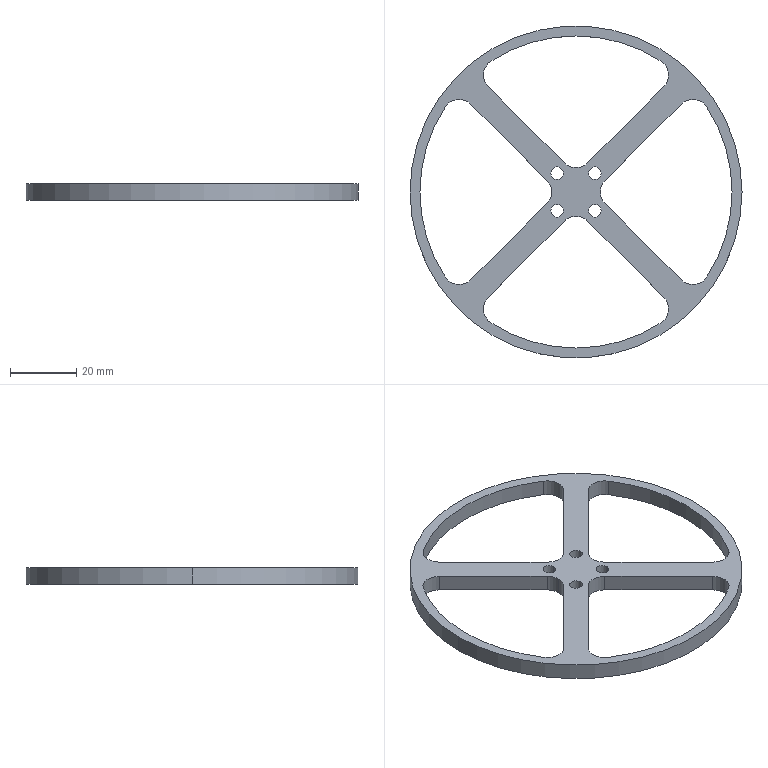Part | SolidWorks | features Cut 1, Extrusion 1, Fillet 1 | 1 solid | 40 faces | box 100 x 100 x 5 mm | volume 11461 mm3 | cylinder 30 | plane 10 | commonest cylinder face diameters 10 x15 3.8 x8 94 x5 100 x2
STEP:
#1=CARTESIAN_POINT('',(-7.557,-5.657,0.));
#2=VERTEX_POINT('',#1);
#3=CARTESIAN_POINT('',(-3.757,-5.657,0.));
#4=VERTEX_POINT('',#3);
#5=CARTESIAN_POINT('',(-5.657,-5.657,0.));
#6=DIRECTION('',(0.,0.,1.));
#7=DIRECTION('',(1.,0.,0.));
#8=AXIS2_PLACEMENT_3D('',#5,#6,#7);
#9=CIRCLE('',#8,1.9);
#10=EDGE_CURVE('',#2,#4,#9,.T.);
#11=ORIENTED_EDGE('',*,*,#10,.F.);
#12=CARTESIAN_POINT('',(-7.557,-5.657,5.));
#13=VERTEX_POINT('',#12);
#14=CARTESIAN_POINT('',(-7.557,-5.657,0.));
#15=DIRECTION('',(0.,0.,1.));
#16=VECTOR('',#15,1000.);
#17=LINE('',#14,#16);
#18=EDGE_CURVE('',#2,#13,#17,.T.);
#19=ORIENTED_EDGE('',*,*,#18,.T.);
#20=CARTESIAN_POINT('',(-3.757,-5.657,5.));
#21=VERTEX_POINT('',#20);
#22=CARTESIAN_POINT('',(-5.657,-5.657,5.));
#23=DIRECTION('',(0.,0.,1.));
#24=DIRECTION('',(1.,0.,0.));
#25=AXIS2_PLACEMENT_3D('',#22,#23,#24);
#26=CIRCLE('',#25,1.9);
#27=EDGE_CURVE('',#13,#21,#26,.T.);
#28=ORIENTED_EDGE('',*,*,#27,.T.);
#29=CARTESIAN_POINT('',(-3.757,-5.657,0.));
#30=DIRECTION('',(0.,0.,1.));
#31=VECTOR('',#30,1000.);
#32=LINE('',#29,#31);
#33=EDGE_CURVE('',#4,#21,#32,.T.);
#34=ORIENTED_EDGE('',*,*,#33,.F.);
#35=EDGE_LOOP('',(#11,#19,#28,#34));
#36=FACE_OUTER_BOUND('',#35,.T.);
#37=CARTESIAN_POINT('',(-5.657,-5.657,0.));
#38=DIRECTION('',(0.,0.,1.));
#39=DIRECTION('',(1.,0.,0.));
#40=AXIS2_PLACEMENT_3D('',#37,#38,#39);
#41=CYLINDRICAL_SURFACE('',#40,1.9);
#42=ADVANCED_FACE('',(#36),#41,.F.);
#43=CARTESIAN_POINT('',(-7.557,5.657,0.));
#44=VERTEX_POINT('',#43);
#45=CARTESIAN_POINT('',(-3.757,5.657,0.));
#46=VERTEX_POINT('',#45);
#47=CARTESIAN_POINT('',(-5.657,5.657,0.));
#48=DIRECTION('',(0.,0.,1.));
#49=DIRECTION('',(1.,0.,0.));
#50=AXIS2_PLACEMENT_3D('',#47,#48,#49);
#51=CIRCLE('',#50,1.9);
#52=EDGE_CURVE('',#44,#46,#51,.T.);
#53=ORIENTED_EDGE('',*,*,#52,.F.);
#54=CARTESIAN_POINT('',(-7.557,5.657,5.));
#55=VERTEX_POINT('',#54);
#56=CARTESIAN_POINT('',(-7.557,5.657,0.));
#57=DIRECTION('',(0.,0.,1.));
#58=VECTOR('',#57,1000.);
#59=LINE('',#56,#58);
#60=EDGE_CURVE('',#44,#55,#59,.T.);
#61=ORIENTED_EDGE('',*,*,#60,.T.);
#62=CARTESIAN_POINT('',(-3.757,5.657,5.));
#63=VERTEX_POINT('',#62);
#64=CARTESIAN_POINT('',(-5.657,5.657,5.));
#65=DIRECTION('',(0.,0.,1.));
#66=DIRECTION('',(1.,0.,0.));
#67=AXIS2_PLACEMENT_3D('',#64,#65,#66);
#68=CIRCLE('',#67,1.9);
#69=EDGE_CURVE('',#55,#63,#68,.T.);
#70=ORIENTED_EDGE('',*,*,#69,.T.);
#71=CARTESIAN_POINT('',(-3.757,5.657,0.));
#72=DIRECTION('',(0.,0.,1.));
#73=VECTOR('',#72,1000.);
#74=LINE('',#71,#73);
#75=EDGE_CURVE('',#46,#63,#74,.T.);
#76=ORIENTED_EDGE('',*,*,#75,.F.);
#77=EDGE_LOOP('',(#53,#61,#70,#76));
#78=FACE_OUTER_BOUND('',#77,.T.);
#79=CARTESIAN_POINT('',(-5.657,5.657,0.));
#80=DIRECTION('',(0.,0.,1.));
#81=DIRECTION('',(1.,0.,0.));
#82=AXIS2_PLACEMENT_3D('',#79,#80,#81);
#83=CYLINDRICAL_SURFACE('',#82,1.9);
#84=ADVANCED_FACE('',(#78),#83,.F.);
#85=CARTESIAN_POINT('',(3.757,5.657,0.));
#86=VERTEX_POINT('',#85);
#87=CARTESIAN_POINT('',(7.557,5.657,0.));
#88=VERTEX_POINT('',#87);
#89=CARTESIAN_POINT('',(5.657,5.657,0.));
#90=DIRECTION('',(0.,0.,1.));
#91=DIRECTION('',(1.,0.,0.));
#92=AXIS2_PLACEMENT_3D('',#89,#90,#91);
#93=CIRCLE('',#92,1.9);
#94=EDGE_CURVE('',#86,#88,#93,.T.);
#95=ORIENTED_EDGE('',*,*,#94,.F.);
#96=CARTESIAN_POINT('',(3.757,5.657,5.));
#97=VERTEX_POINT('',#96);
#98=CARTESIAN_POINT('',(3.757,5.657,0.));
#99=DIRECTION('',(0.,0.,1.));
#100=VECTOR('',#99,1000.);
#101=LINE('',#98,#100);
#102=EDGE_CURVE('',#86,#97,#101,.T.);
#103=ORIENTED_EDGE('',*,*,#102,.T.);
#104=CARTESIAN_POINT('',(7.557,5.657,5.));
#105=VERTEX_POINT('',#104);
#106=CARTESIAN_POINT('',(5.657,5.657,5.));
#107=DIRECTION('',(0.,0.,1.));
#108=DIRECTION('',(1.,0.,0.));
#109=AXIS2_PLACEMENT_3D('',#106,#107,#108);
#110=CIRCLE('',#109,1.9);
#111=EDGE_CURVE('',#97,#105,#110,.T.);
#112=ORIENTED_EDGE('',*,*,#111,.T.);
#113=CARTESIAN_POINT('',(7.557,5.657,0.));
#114=DIRECTION('',(0.,0.,1.));
#115=VECTOR('',#114,1000.);
#116=LINE('',#113,#115);
#117=EDGE_CURVE('',#88,#105,#116,.T.);
#118=ORIENTED_EDGE('',*,*,#117,.F.);
#119=EDGE_LOOP('',(#95,#103,#112,#118));
#120=FACE_OUTER_BOUND('',#119,.T.);
#121=CARTESIAN_POINT('',(5.657,5.657,0.));
#122=DIRECTION('',(0.,0.,1.));
#123=DIRECTION('',(1.,0.,0.));
#124=AXIS2_PLACEMENT_3D('',#121,#122,#123);
#125=CYLINDRICAL_SURFACE('',#124,1.9);
#126=ADVANCED_FACE('',(#120),#125,.F.);
#127=CARTESIAN_POINT('',(3.757,-5.657,0.));
#128=VERTEX_POINT('',#127);
#129=CARTESIAN_POINT('',(7.557,-5.657,0.));
#130=VERTEX_POINT('',#129);
#131=CARTESIAN_POINT('',(5.657,-5.657,0.));
#132=DIRECTION('',(0.,0.,1.));
#133=DIRECTION('',(1.,0.,0.));
#134=AXIS2_PLACEMENT_3D('',#131,#132,#133);
#135=CIRCLE('',#134,1.9);
#136=EDGE_CURVE('',#128,#130,#135,.T.);
#137=ORIENTED_EDGE('',*,*,#136,.F.);
#138=CARTESIAN_POINT('',(3.757,-5.657,5.));
#139=VERTEX_POINT('',#138);
#140=CARTESIAN_POINT('',(3.757,-5.657,0.));
#141=DIRECTION('',(0.,0.,1.));
#142=VECTOR('',#141,1000.);
#143=LINE('',#140,#142);
#144=EDGE_CURVE('',#128,#139,#143,.T.);
#145=ORIENTED_EDGE('',*,*,#144,.T.);
#146=CARTESIAN_POINT('',(7.557,-5.657,5.));
#147=VERTEX_POINT('',#146);
#148=CARTESIAN_POINT('',(5.657,-5.657,5.));
#149=DIRECTION('',(0.,0.,1.));
#150=DIRECTION('',(1.,0.,0.));
#151=AXIS2_PLACEMENT_3D('',#148,#149,#150);
#152=CIRCLE('',#151,1.9);
#153=EDGE_CURVE('',#139,#147,#152,.T.);
#154=ORIENTED_EDGE('',*,*,#153,.T.);
#155=CARTESIAN_POINT('',(7.557,-5.657,0.));
#156=DIRECTION('',(0.,0.,1.));
#157=VECTOR('',#156,1000.);
#158=LINE('',#155,#157);
#159=EDGE_CURVE('',#130,#147,#158,.T.);
#160=ORIENTED_EDGE('',*,*,#159,.F.);
#161=EDGE_LOOP('',(#137,#145,#154,#160));
#162=FACE_OUTER_BOUND('',#161,.T.);
#163=CARTESIAN_POINT('',(5.657,-5.657,0.));
#164=DIRECTION('',(0.,0.,1.));
#165=DIRECTION('',(1.,0.,0.));
#166=AXIS2_PLACEMENT_3D('',#163,#164,#165);
#167=CYLINDRICAL_SURFACE('',#166,1.9);
#168=ADVANCED_FACE('',(#162),#167,.F.);
#169=CARTESIAN_POINT('',(-27.891,35.214,5.));
#170=VERTEX_POINT('',#169);
#171=CARTESIAN_POINT('',(-25.616,39.406,5.));
#172=VERTEX_POINT('',#171);
#173=CARTESIAN_POINT('',(-22.891,35.214,5.));
#174=DIRECTION('',(0.,0.,-1.));
#175=DIRECTION('',(1.,0.,0.));
#176=AXIS2_PLACEMENT_3D('',#173,#174,#175);
#177=CIRCLE('',#176,5.);
#178=EDGE_CURVE('',#170,#172,#177,.T.);
#179=ORIENTED_EDGE('',*,*,#178,.F.);
#180=CARTESIAN_POINT('',(-27.891,35.214,0.));
#181=VERTEX_POINT('',#180);
#182=CARTESIAN_POINT('',(-27.891,35.214,5.));
#183=DIRECTION('',(0.,0.,-1.));
#184=VECTOR('',#183,1000.);
#185=LINE('',#182,#184);
#186=EDGE_CURVE('',#170,#181,#185,.T.);
#187=ORIENTED_EDGE('',*,*,#186,.T.);
#188=CARTESIAN_POINT('',(-25.616,39.406,0.));
#189=VERTEX_POINT('',#188);
#190=CARTESIAN_POINT('',(-22.891,35.214,0.));
#191=DIRECTION('',(0.,0.,1.));
#192=DIRECTION('',(1.,0.,0.));
#193=AXIS2_PLACEMENT_3D('',#190,#191,#192);
#194=CIRCLE('',#193,5.);
#195=EDGE_CURVE('',#189,#181,#194,.T.);
#196=ORIENTED_EDGE('',*,*,#195,.F.);
#197=CARTESIAN_POINT('',(-25.616,39.406,5.));
#198=DIRECTION('',(0.,0.,-1.));
#199=VECTOR('',#198,1000.);
#200=LINE('',#197,#199);
#201=EDGE_CURVE('',#172,#189,#200,.T.);
#202=ORIENTED_EDGE('',*,*,#201,.F.);
#203=EDGE_LOOP('',(#179,#187,#196,#202));
#204=FACE_OUTER_BOUND('',#203,.T.);
#205=CARTESIAN_POINT('',(-22.891,35.214,5.));
#206=DIRECTION('',(0.,0.,-1.));
#207=DIRECTION('',(-1.,0.,0.));
#208=AXIS2_PLACEMENT_3D('',#205,#206,#207);
#209=CYLINDRICAL_SURFACE('',#208,5.);
#210=ADVANCED_FACE('',(#204),#209,.F.);
#211=CARTESIAN_POINT('',(-27.891,-35.214,5.));
#212=VERTEX_POINT('',#211);
#213=CARTESIAN_POINT('',(-26.427,-31.678,5.));
#214=VERTEX_POINT('',#213);
#215=CARTESIAN_POINT('',(-22.891,-35.214,5.));
#216=DIRECTION('',(0.,0.,-1.));
#217=DIRECTION('',(1.,0.,0.));
#218=AXIS2_PLACEMENT_3D('',#215,#216,#217);
#219=CIRCLE('',#218,5.);
#220=EDGE_CURVE('',#212,#214,#219,.T.);
#221=ORIENTED_EDGE('',*,*,#220,.F.);
#222=CARTESIAN_POINT('',(-27.891,-35.214,0.));
#223=VERTEX_POINT('',#222);
#224=CARTESIAN_POINT('',(-27.891,-35.214,5.));
#225=DIRECTION('',(0.,0.,-1.));
#226=VECTOR('',#225,1000.);
#227=LINE('',#224,#226);
#228=EDGE_CURVE('',#212,#223,#227,.T.);
#229=ORIENTED_EDGE('',*,*,#228,.T.);
#230=CARTESIAN_POINT('',(-26.427,-31.678,0.));
#231=VERTEX_POINT('',#230);
#232=CARTESIAN_POINT('',(-22.891,-35.214,0.));
#233=DIRECTION('',(0.,0.,1.));
#234=DIRECTION('',(1.,0.,0.));
#235=AXIS2_PLACEMENT_3D('',#232,#233,#234);
#236=CIRCLE('',#235,5.);
#237=EDGE_CURVE('',#231,#223,#236,.T.);
#238=ORIENTED_EDGE('',*,*,#237,.F.);
#239=CARTESIAN_POINT('',(-26.427,-31.678,0.));
#240=DIRECTION('',(0.,0.,-1.));
#241=VECTOR('',#240,1000.);
#242=LINE('',#239,#241);
#243=EDGE_CURVE('',#214,#231,#242,.T.);
#244=ORIENTED_EDGE('',*,*,#243,.F.);
#245=EDGE_LOOP('',(#221,#229,#238,#244));
#246=FACE_OUTER_BOUND('',#245,.T.);
#247=CARTESIAN_POINT('',(-22.891,-35.214,5.));
#248=DIRECTION('',(0.,0.,-1.));
#249=DIRECTION('',(-1.,0.,0.));
#250=AXIS2_PLACEMENT_3D('',#247,#248,#249);
#251=CYLINDRICAL_SURFACE('',#250,5.);
#252=ADVANCED_FACE('',(#246),#251,.F.);
#253=CARTESIAN_POINT('',(-7.322,0.,0.));
#254=VERTEX_POINT('',#253);
#255=CARTESIAN_POINT('',(-8.787,3.536,0.));
#256=VERTEX_POINT('',#255);
#257=CARTESIAN_POINT('',(-12.322,0.,0.));
#258=DIRECTION('',(0.,0.,1.));
#259=DIRECTION('',(1.,0.,0.));
#260=AXIS2_PLACEMENT_3D('',#257,#258,#259);
#261=CIRCLE('',#260,5.);
#262=EDGE_CURVE('',#254,#256,#261,.T.);
#263=ORIENTED_EDGE('',*,*,#262,.F.);
#264=CARTESIAN_POINT('',(-7.322,0.,5.));
#265=VERTEX_POINT('',#264);
#266=CARTESIAN_POINT('',(-7.322,0.,5.));
#267=DIRECTION('',(0.,0.,1.));
#268=VECTOR('',#267,1000.);
#269=LINE('',#266,#268);
#270=EDGE_CURVE('',#254,#265,#269,.T.);
#271=ORIENTED_EDGE('',*,*,#270,.T.);
#272=CARTESIAN_POINT('',(-8.787,3.536,5.));
#273=VERTEX_POINT('',#272);
#274=CARTESIAN_POINT('',(-12.322,0.,5.));
#275=DIRECTION('',(0.,0.,-1.));
#276=DIRECTION('',(1.,0.,0.));
#277=AXIS2_PLACEMENT_3D('',#274,#275,#276);
#278=CIRCLE('',#277,5.);
#279=EDGE_CURVE('',#273,#265,#278,.T.);
#280=ORIENTED_EDGE('',*,*,#279,.F.);
#281=CARTESIAN_POINT('',(-8.787,3.536,5.));
#282=DIRECTION('',(0.,0.,1.));
#283=VECTOR('',#282,1000.);
#284=LINE('',#281,#283);
#285=EDGE_CURVE('',#256,#273,#284,.T.);
#286=ORIENTED_EDGE('',*,*,#285,.F.);
#287=EDGE_LOOP('',(#263,#271,#280,#286));
#288=FACE_OUTER_BOUND('',#287,.T.);
#289=CARTESIAN_POINT('',(-12.322,0.,5.));
#290=DIRECTION('',(0.,0.,1.));
#291=DIRECTION('',(1.,0.,0.));
#292=AXIS2_PLACEMENT_3D('',#289,#290,#291);
#293=CYLINDRICAL_SURFACE('',#292,5.);
#294=ADVANCED_FACE('',(#288),#293,.F.);
#295=CARTESIAN_POINT('',(-39.406,25.616,5.));
#296=VERTEX_POINT('',#295);
#297=CARTESIAN_POINT('',(-47.,0.,5.));
#298=VERTEX_POINT('',#297);
#299=CARTESIAN_POINT('',(0.,0.,5.));
#300=DIRECTION('',(0.,0.,1.));
#301=DIRECTION('',(1.,0.,0.));
#302=AXIS2_PLACEMENT_3D('',#299,#300,#301);
#303=CIRCLE('',#302,47.);
#304=EDGE_CURVE('',#296,#298,#303,.T.);
#305=ORIENTED_EDGE('',*,*,#304,.T.);
#306=CARTESIAN_POINT('',(-47.,0.,0.));
#307=VERTEX_POINT('',#306);
#308=CARTESIAN_POINT('',(-47.,0.,5.));
#309=DIRECTION('',(0.,0.,-1.));
#310=VECTOR('',#309,1000.);
#311=LINE('',#308,#310);
#312=EDGE_CURVE('',#298,#307,#311,.T.);
#313=ORIENTED_EDGE('',*,*,#312,.T.);
#314=CARTESIAN_POINT('',(-39.406,25.616,0.));
#315=VERTEX_POINT('',#314);
#316=CARTESIAN_POINT('',(0.,0.,0.));
#317=DIRECTION('',(0.,0.,1.));
#318=DIRECTION('',(1.,0.,0.));
#319=AXIS2_PLACEMENT_3D('',#316,#317,#318);
#320=CIRCLE('',#319,47.);
#321=EDGE_CURVE('',#315,#307,#320,.T.);
#322=ORIENTED_EDGE('',*,*,#321,.F.);
#323=CARTESIAN_POINT('',(-39.406,25.616,5.));
#324=DIRECTION('',(0.,0.,1.));
#325=VECTOR('',#324,1000.);
#326=LINE('',#323,#325);
#327=EDGE_CURVE('',#315,#296,#326,.T.);
#328=ORIENTED_EDGE('',*,*,#327,.T.);
#329=EDGE_LOOP('',(#305,#313,#322,#328));
#330=FACE_OUTER_BOUND('',#329,.T.);
#331=CARTESIAN_POINT('',(0.,0.,5.));
#332=DIRECTION('',(0.,0.,-1.));
#333=DIRECTION('',(-1.,0.,0.));
#334=AXIS2_PLACEMENT_3D('',#331,#332,#333);
#335=CYLINDRICAL_SURFACE('',#334,47.);
#336=ADVANCED_FACE('',(#330),#335,.F.);
#337=CARTESIAN_POINT('',(50.,0.,5.));
#338=VERTEX_POINT('',#337);
#339=CARTESIAN_POINT('',(-50.,0.,5.));
#340=VERTEX_POINT('',#339);
#341=CARTESIAN_POINT('',(0.,0.,5.));
#342=DIRECTION('',(0.,0.,1.));
#343=DIRECTION('',(1.,0.,0.));
#344=AXIS2_PLACEMENT_3D('',#341,#342,#343);
#345=CIRCLE('',#344,50.);
#346=EDGE_CURVE('',#338,#340,#345,.T.);
#347=ORIENTED_EDGE('',*,*,#346,.F.);
#348=CARTESIAN_POINT('',(50.,0.,0.));
#349=VERTEX_POINT('',#348);
#350=CARTESIAN_POINT('',(50.,0.,5.));
#351=DIRECTION('',(0.,0.,-1.));
#352=VECTOR('',#351,1000.);
#353=LINE('',#350,#352);
#354=EDGE_CURVE('',#338,#349,#353,.T.);
#355=ORIENTED_EDGE('',*,*,#354,.T.);
#356=CARTESIAN_POINT('',(-50.,0.,0.));
#357=VERTEX_POINT('',#356);
#358=CARTESIAN_POINT('',(0.,0.,0.));
#359=DIRECTION('',(0.,0.,1.));
#360=DIRECTION('',(1.,0.,0.));
#361=AXIS2_PLACEMENT_3D('',#358,#359,#360);
#362=CIRCLE('',#361,50.);
#363=EDGE_CURVE('',#349,#357,#362,.T.);
#364=ORIENTED_EDGE('',*,*,#363,.T.);
#365=CARTESIAN_POINT('',(-50.,0.,5.));
#366=DIRECTION('',(0.,0.,-1.));
#367=VECTOR('',#366,1000.);
#368=LINE('',#365,#367);
#369=EDGE_CURVE('',#340,#357,#368,.T.);
#370=ORIENTED_EDGE('',*,*,#369,.F.);
#371=EDGE_LOOP('',(#347,#355,#364,#370));
#372=FACE_OUTER_BOUND('',#371,.T.);
#373=CARTESIAN_POINT('',(0.,0.,5.));
#374=DIRECTION('',(0.,0.,-1.));
#375=DIRECTION('',(-1.,0.,0.));
#376=AXIS2_PLACEMENT_3D('',#373,#374,#375);
#377=CYLINDRICAL_SURFACE('',#376,50.);
#378=ADVANCED_FACE('',(#372),#377,.T.);
#379=CARTESIAN_POINT('',(-5.657,-5.657,5.));
#380=DIRECTION('',(0.,0.,1.));
#381=DIRECTION('',(1.,0.,0.));
#382=AXIS2_PLACEMENT_3D('',#379,#380,#381);
#383=CIRCLE('',#382,1.9);
#384=EDGE_CURVE('',#21,#13,#383,.T.);
#385=ORIENTED_EDGE('',*,*,#384,.F.);
#386=ORIENTED_EDGE('',*,*,#27,.F.);
#387=EDGE_LOOP('',(#385,#386));
#388=FACE_BOUND('',#387,.T.);
#389=CARTESIAN_POINT('',(-5.657,5.657,5.));
#390=DIRECTION('',(0.,0.,1.));
#391=DIRECTION('',(1.,0.,0.));
#392=AXIS2_PLACEMENT_3D('',#389,#390,#391);
#393=CIRCLE('',#392,1.9);
#394=EDGE_CURVE('',#63,#55,#393,.T.);
#395=ORIENTED_EDGE('',*,*,#394,.F.);
#396=ORIENTED_EDGE('',*,*,#69,.F.);
#397=EDGE_LOOP('',(#395,#396));
#398=FACE_BOUND('',#397,.T.);
#399=CARTESIAN_POINT('',(5.657,5.657,5.));
#400=DIRECTION('',(0.,0.,1.));
#401=DIRECTION('',(1.,0.,0.));
#402=AXIS2_PLACEMENT_3D('',#399,#400,#401);
#403=CIRCLE('',#402,1.9);
#404=EDGE_CURVE('',#105,#97,#403,.T.);
#405=ORIENTED_EDGE('',*,*,#404,.F.);
#406=ORIENTED_EDGE('',*,*,#111,.F.);
#407=EDGE_LOOP('',(#405,#406));
#408=FACE_BOUND('',#407,.T.);
#409=CARTESIAN_POINT('',(5.657,-5.657,5.));
#410=DIRECTION('',(0.,0.,1.));
#411=DIRECTION('',(1.,0.,0.));
#412=AXIS2_PLACEMENT_3D('',#409,#410,#411);
#413=CIRCLE('',#412,1.9);
#414=EDGE_CURVE('',#147,#139,#413,.T.);
#415=ORIENTED_EDGE('',*,*,#414,.F.);
#416=ORIENTED_EDGE('',*,*,#153,.F.);
#417=EDGE_LOOP('',(#415,#416));
#418=FACE_BOUND('',#417,.T.);
#419=CARTESIAN_POINT('',(31.678,26.427,5.));
#420=VERTEX_POINT('',#419);
#421=CARTESIAN_POINT('',(8.787,3.536,5.));
#422=VERTEX_POINT('',#421);
#423=CARTESIAN_POINT('',(5.251,0.,5.));
#424=DIRECTION('',(-0.7071,-0.7071,0.));
#425=VECTOR('',#424,1000.);
#426=LINE('',#423,#425);
#427=EDGE_CURVE('',#420,#422,#426,.T.);
#428=ORIENTED_EDGE('',*,*,#427,.F.);
#429=CARTESIAN_POINT('',(39.406,25.616,5.));
#430=VERTEX_POINT('',#429);
#431=CARTESIAN_POINT('',(35.214,22.891,5.));
#432=DIRECTION('',(0.,0.,-1.));
#433=DIRECTION('',(1.,0.,0.));
#434=AXIS2_PLACEMENT_3D('',#431,#432,#433);
#435=CIRCLE('',#434,5.);
#436=EDGE_CURVE('',#420,#430,#435,.T.);
#437=ORIENTED_EDGE('',*,*,#436,.T.);
#438=CARTESIAN_POINT('',(39.406,-25.616,5.));
#439=VERTEX_POINT('',#438);
#440=CARTESIAN_POINT('',(0.,0.,5.));
#441=DIRECTION('',(0.,0.,1.));
#442=DIRECTION('',(1.,0.,0.));
#443=AXIS2_PLACEMENT_3D('',#440,#441,#442);
#444=CIRCLE('',#443,47.);
#445=EDGE_CURVE('',#439,#430,#444,.T.);
#446=ORIENTED_EDGE('',*,*,#445,.F.);
#447=CARTESIAN_POINT('',(31.678,-26.427,5.));
#448=VERTEX_POINT('',#447);
#449=CARTESIAN_POINT('',(35.214,-22.891,5.));
#450=DIRECTION('',(0.,0.,-1.));
#451=DIRECTION('',(1.,0.,0.));
#452=AXIS2_PLACEMENT_3D('',#449,#450,#451);
#453=CIRCLE('',#452,5.);
#454=EDGE_CURVE('',#439,#448,#453,.T.);
#455=ORIENTED_EDGE('',*,*,#454,.T.);
#456=CARTESIAN_POINT('',(8.787,-3.536,5.));
#457=VERTEX_POINT('',#456);
#458=CARTESIAN_POINT('',(5.251,0.,5.));
#459=DIRECTION('',(0.7071,-0.7071,0.));
#460=VECTOR('',#459,1000.);
#461=LINE('',#458,#460);
#462=EDGE_CURVE('',#457,#448,#461,.T.);
#463=ORIENTED_EDGE('',*,*,#462,.F.);
#464=CARTESIAN_POINT('',(12.322,0.,5.));
#465=DIRECTION('',(0.,0.,-1.));
#466=DIRECTION('',(1.,0.,0.));
#467=AXIS2_PLACEMENT_3D('',#464,#465,#466);
#468=CIRCLE('',#467,5.);
#469=EDGE_CURVE('',#457,#422,#468,.T.);
#470=ORIENTED_EDGE('',*,*,#469,.T.);
#471=EDGE_LOOP('',(#428,#437,#446,#455,#463,#470));
#472=FACE_BOUND('',#471,.T.);
#473=CARTESIAN_POINT('',(-26.427,31.678,5.));
#474=VERTEX_POINT('',#473);
#475=CARTESIAN_POINT('',(-3.536,8.787,5.));
#476=VERTEX_POINT('',#475);
#477=CARTESIAN_POINT('',(-30.505,35.756,5.));
#478=DIRECTION('',(0.7071,-0.7071,0.));
#479=VECTOR('',#478,1000.);
#480=LINE('',#477,#479);
#481=EDGE_CURVE('',#474,#476,#480,.T.);
#482=ORIENTED_EDGE('',*,*,#481,.F.);
#483=CARTESIAN_POINT('',(-22.891,35.214,5.));
#484=DIRECTION('',(0.,0.,-1.));
#485=DIRECTION('',(1.,0.,0.));
#486=AXIS2_PLACEMENT_3D('',#483,#484,#485);
#487=CIRCLE('',#486,5.);
#488=EDGE_CURVE('',#474,#170,#487,.T.);
#489=ORIENTED_EDGE('',*,*,#488,.T.);
#490=ORIENTED_EDGE('',*,*,#178,.T.);
#491=CARTESIAN_POINT('',(25.616,39.406,5.));
#492=VERTEX_POINT('',#491);
#493=CARTESIAN_POINT('',(0.,0.,5.));
#494=DIRECTION('',(0.,0.,1.));
#495=DIRECTION('',(1.,0.,0.));
#496=AXIS2_PLACEMENT_3D('',#493,#494,#495);
#497=CIRCLE('',#496,47.);
#498=EDGE_CURVE('',#492,#172,#497,.T.);
#499=ORIENTED_EDGE('',*,*,#498,.F.);
#500=CARTESIAN_POINT('',(26.427,31.678,5.));
#501=VERTEX_POINT('',#500);
#502=CARTESIAN_POINT('',(22.891,35.214,5.));
#503=DIRECTION('',(0.,0.,-1.));
#504=DIRECTION('',(1.,0.,0.));
#505=AXIS2_PLACEMENT_3D('',#502,#503,#504);
#506=CIRCLE('',#505,5.);
#507=EDGE_CURVE('',#492,#501,#506,.T.);
#508=ORIENTED_EDGE('',*,*,#507,.T.);
#509=CARTESIAN_POINT('',(3.536,8.787,5.));
#510=VERTEX_POINT('',#509);
#511=CARTESIAN_POINT('',(30.505,35.756,5.));
#512=DIRECTION('',(0.7071,0.7071,0.));
#513=VECTOR('',#512,1000.);
#514=LINE('',#511,#513);
#515=EDGE_CURVE('',#510,#501,#514,.T.);
#516=ORIENTED_EDGE('',*,*,#515,.F.);
#517=CARTESIAN_POINT('',(0.,12.322,5.));
#518=DIRECTION('',(0.,0.,-1.));
#519=DIRECTION('',(1.,0.,0.));
#520=AXIS2_PLACEMENT_3D('',#517,#518,#519);
#521=CIRCLE('',#520,5.);
#522=EDGE_CURVE('',#510,#476,#521,.T.);
#523=ORIENTED_EDGE('',*,*,#522,.T.);
#524=EDGE_LOOP('',(#482,#489,#490,#499,#508,#516,#523));
#525=FACE_BOUND('',#524,.T.);
#526=CARTESIAN_POINT('',(0.,0.,5.));
#527=DIRECTION('',(0.,0.,1.));
#528=DIRECTION('',(1.,0.,0.));
#529=AXIS2_PLACEMENT_3D('',#526,#527,#528);
#530=CIRCLE('',#529,50.);
#531=EDGE_CURVE('',#340,#338,#530,.T.);
#532=ORIENTED_EDGE('',*,*,#531,.T.);
#533=ORIENTED_EDGE('',*,*,#346,.T.);
#534=EDGE_LOOP('',(#532,#533));
#535=FACE_OUTER_BOUND('',#534,.T.);
#536=ORIENTED_EDGE('',*,*,#304,.F.);
#537=CARTESIAN_POINT('',(-31.678,26.427,5.));
#538=VERTEX_POINT('',#537);
#539=CARTESIAN_POINT('',(-35.214,22.891,5.));
#540=DIRECTION('',(0.,0.,-1.));
#541=DIRECTION('',(1.,0.,0.));
#542=AXIS2_PLACEMENT_3D('',#539,#540,#541);
#543=CIRCLE('',#542,5.);
#544=EDGE_CURVE('',#296,#538,#543,.T.);
#545=ORIENTED_EDGE('',*,*,#544,.T.);
#546=CARTESIAN_POINT('',(-5.251,0.,5.));
#547=DIRECTION('',(-0.7071,0.7071,0.));
#548=VECTOR('',#547,1000.);
#549=LINE('',#546,#548);
#550=EDGE_CURVE('',#273,#538,#549,.T.);
#551=ORIENTED_EDGE('',*,*,#550,.F.);
#552=ORIENTED_EDGE('',*,*,#279,.T.);
#553=CARTESIAN_POINT('',(-8.787,-3.536,5.));
#554=VERTEX_POINT('',#553);
#555=CARTESIAN_POINT('',(-12.322,0.,5.));
#556=DIRECTION('',(0.,0.,-1.));
#557=DIRECTION('',(1.,0.,0.));
#558=AXIS2_PLACEMENT_3D('',#555,#556,#557);
#559=CIRCLE('',#558,5.);
#560=EDGE_CURVE('',#265,#554,#559,.T.);
#561=ORIENTED_EDGE('',*,*,#560,.T.);
#562=CARTESIAN_POINT('',(-31.678,-26.427,5.));
#563=VERTEX_POINT('',#562);
#564=CARTESIAN_POINT('',(-5.251,0.,5.));
#565=DIRECTION('',(0.7071,0.7071,0.));
#566=VECTOR('',#565,1000.);
#567=LINE('',#564,#566);
#568=EDGE_CURVE('',#563,#554,#567,.T.);
#569=ORIENTED_EDGE('',*,*,#568,.F.);
#570=CARTESIAN_POINT('',(-39.406,-25.616,5.));
#571=VERTEX_POINT('',#570);
#572=CARTESIAN_POINT('',(-35.214,-22.891,5.));
#573=DIRECTION('',(0.,0.,-1.));
#574=DIRECTION('',(1.,0.,0.));
#575=AXIS2_PLACEMENT_3D('',#572,#573,#574);
#576=CIRCLE('',#575,5.);
#577=EDGE_CURVE('',#563,#571,#576,.T.);
#578=ORIENTED_EDGE('',*,*,#577,.T.);
#579=CARTESIAN_POINT('',(0.,0.,5.));
#580=DIRECTION('',(0.,0.,1.));
#581=DIRECTION('',(1.,0.,0.));
#582=AXIS2_PLACEMENT_3D('',#579,#580,#581);
#583=CIRCLE('',#582,47.);
#584=EDGE_CURVE('',#298,#571,#583,.T.);
#585=ORIENTED_EDGE('',*,*,#584,.F.);
#586=EDGE_LOOP('',(#536,#545,#551,#552,#561,#569,#578,#585));
#587=FACE_BOUND('',#586,.T.);
#588=CARTESIAN_POINT('',(26.427,-31.678,5.));
#589=VERTEX_POINT('',#588);
#590=CARTESIAN_POINT('',(3.536,-8.787,5.));
#591=VERTEX_POINT('',#590);
#592=CARTESIAN_POINT('',(0.,-5.251,5.));
#593=DIRECTION('',(-0.7071,0.7071,0.));
#594=VECTOR('',#593,1000.);
#595=LINE('',#592,#594);
#596=EDGE_CURVE('',#589,#591,#595,.T.);
#597=ORIENTED_EDGE('',*,*,#596,.F.);
#598=CARTESIAN_POINT('',(25.616,-39.406,5.));
#599=VERTEX_POINT('',#598);
#600=CARTESIAN_POINT('',(22.891,-35.214,5.));
#601=DIRECTION('',(0.,0.,-1.));
#602=DIRECTION('',(1.,0.,0.));
#603=AXIS2_PLACEMENT_3D('',#600,#601,#602);
#604=CIRCLE('',#603,5.);
#605=EDGE_CURVE('',#589,#599,#604,.T.);
#606=ORIENTED_EDGE('',*,*,#605,.T.);
#607=CARTESIAN_POINT('',(-25.616,-39.406,5.));
#608=VERTEX_POINT('',#607);
#609=CARTESIAN_POINT('',(0.,0.,5.));
#610=DIRECTION('',(0.,0.,1.));
#611=DIRECTION('',(1.,0.,0.));
#612=AXIS2_PLACEMENT_3D('',#609,#610,#611);
#613=CIRCLE('',#612,47.);
#614=EDGE_CURVE('',#608,#599,#613,.T.);
#615=ORIENTED_EDGE('',*,*,#614,.F.);
#616=CARTESIAN_POINT('',(-22.891,-35.214,5.));
#617=DIRECTION('',(0.,0.,-1.));
#618=DIRECTION('',(1.,0.,0.));
#619=AXIS2_PLACEMENT_3D('',#616,#617,#618);
#620=CIRCLE('',#619,5.);
#621=EDGE_CURVE('',#608,#212,#620,.T.);
#622=ORIENTED_EDGE('',*,*,#621,.T.);
#623=ORIENTED_EDGE('',*,*,#220,.T.);
#624=CARTESIAN_POINT('',(-3.536,-8.787,5.));
#625=VERTEX_POINT('',#624);
#626=CARTESIAN_POINT('',(0.,-5.251,5.));
#627=DIRECTION('',(-0.7071,-0.7071,0.));
#628=VECTOR('',#627,1000.);
#629=LINE('',#626,#628);
#630=EDGE_CURVE('',#625,#214,#629,.T.);
#631=ORIENTED_EDGE('',*,*,#630,.F.);
#632=CARTESIAN_POINT('',(0.,-12.322,5.));
#633=DIRECTION('',(0.,0.,-1.));
#634=DIRECTION('',(1.,0.,0.));
#635=AXIS2_PLACEMENT_3D('',#632,#633,#634);
#636=CIRCLE('',#635,5.);
#637=EDGE_CURVE('',#625,#591,#636,.T.);
#638=ORIENTED_EDGE('',*,*,#637,.T.);
#639=EDGE_LOOP('',(#597,#606,#615,#622,#623,#631,#638));
#640=FACE_BOUND('',#639,.T.);
#641=CARTESIAN_POINT('',(0.,0.,5.));
#642=DIRECTION('',(0.,0.,1.));
#643=DIRECTION('',(1.,0.,0.));
#644=AXIS2_PLACEMENT_3D('',#641,#642,#643);
#645=PLANE('',#644);
#646=ADVANCED_FACE('',(#388,#398,#408,#418,#472,#525,#535,#587,#640),#645,.T.);
#647=CARTESIAN_POINT('',(-5.657,-5.657,0.));
#648=DIRECTION('',(0.,0.,1.));
#649=DIRECTION('',(1.,0.,0.));
#650=AXIS2_PLACEMENT_3D('',#647,#648,#649);
#651=CIRCLE('',#650,1.9);
#652=EDGE_CURVE('',#4,#2,#651,.T.);
#653=ORIENTED_EDGE('',*,*,#652,.T.);
#654=ORIENTED_EDGE('',*,*,#10,.T.);
#655=EDGE_LOOP('',(#653,#654));
#656=FACE_BOUND('',#655,.T.);
#657=CARTESIAN_POINT('',(-5.657,5.657,0.));
#658=DIRECTION('',(0.,0.,1.));
#659=DIRECTION('',(1.,0.,0.));
#660=AXIS2_PLACEMENT_3D('',#657,#658,#659);
#661=CIRCLE('',#660,1.9);
#662=EDGE_CURVE('',#46,#44,#661,.T.);
#663=ORIENTED_EDGE('',*,*,#662,.T.);
#664=ORIENTED_EDGE('',*,*,#52,.T.);
#665=EDGE_LOOP('',(#663,#664));
#666=FACE_BOUND('',#665,.T.);
#667=CARTESIAN_POINT('',(5.657,5.657,0.));
#668=DIRECTION('',(0.,0.,1.));
#669=DIRECTION('',(1.,0.,0.));
#670=AXIS2_PLACEMENT_3D('',#667,#668,#669);
#671=CIRCLE('',#670,1.9);
#672=EDGE_CURVE('',#88,#86,#671,.T.);
#673=ORIENTED_EDGE('',*,*,#672,.T.);
#674=ORIENTED_EDGE('',*,*,#94,.T.);
#675=EDGE_LOOP('',(#673,#674));
#676=FACE_BOUND('',#675,.T.);
#677=CARTESIAN_POINT('',(5.657,-5.657,0.));
#678=DIRECTION('',(0.,0.,1.));
#679=DIRECTION('',(1.,0.,0.));
#680=AXIS2_PLACEMENT_3D('',#677,#678,#679);
#681=CIRCLE('',#680,1.9);
#682=EDGE_CURVE('',#130,#128,#681,.T.);
#683=ORIENTED_EDGE('',*,*,#682,.T.);
#684=ORIENTED_EDGE('',*,*,#136,.T.);
#685=EDGE_LOOP('',(#683,#684));
#686=FACE_BOUND('',#685,.T.);
#687=CARTESIAN_POINT('',(8.787,-3.536,0.));
#688=VERTEX_POINT('',#687);
#689=CARTESIAN_POINT('',(31.678,-26.427,0.));
#690=VERTEX_POINT('',#689);
#691=CARTESIAN_POINT('',(5.251,0.,0.));
#692=DIRECTION('',(0.7071,-0.7071,0.));
#693=VECTOR('',#692,1000.);
#694=LINE('',#691,#693);
#695=EDGE_CURVE('',#688,#690,#694,.T.);
#696=ORIENTED_EDGE('',*,*,#695,.T.);
#697=CARTESIAN_POINT('',(39.406,-25.616,0.));
#698=VERTEX_POINT('',#697);
#699=CARTESIAN_POINT('',(35.214,-22.891,0.));
#700=DIRECTION('',(0.,0.,1.));
#701=DIRECTION('',(1.,0.,0.));
#702=AXIS2_PLACEMENT_3D('',#699,#700,#701);
#703=CIRCLE('',#702,5.);
#704=EDGE_CURVE('',#690,#698,#703,.T.);
#705=ORIENTED_EDGE('',*,*,#704,.T.);
#706=CARTESIAN_POINT('',(39.406,25.616,0.));
#707=VERTEX_POINT('',#706);
#708=CARTESIAN_POINT('',(0.,0.,0.));
#709=DIRECTION('',(0.,0.,1.));
#710=DIRECTION('',(1.,0.,0.));
#711=AXIS2_PLACEMENT_3D('',#708,#709,#710);
#712=CIRCLE('',#711,47.);
#713=EDGE_CURVE('',#698,#707,#712,.T.);
#714=ORIENTED_EDGE('',*,*,#713,.T.);
#715=CARTESIAN_POINT('',(31.678,26.427,0.));
#716=VERTEX_POINT('',#715);
#717=CARTESIAN_POINT('',(35.214,22.891,0.));
#718=DIRECTION('',(0.,0.,1.));
#719=DIRECTION('',(1.,0.,0.));
#720=AXIS2_PLACEMENT_3D('',#717,#718,#719);
#721=CIRCLE('',#720,5.);
#722=EDGE_CURVE('',#707,#716,#721,.T.);
#723=ORIENTED_EDGE('',*,*,#722,.T.);
#724=CARTESIAN_POINT('',(8.787,3.536,0.));
#725=VERTEX_POINT('',#724);
#726=CARTESIAN_POINT('',(5.251,0.,0.));
#727=DIRECTION('',(-0.7071,-0.7071,0.));
#728=VECTOR('',#727,1000.);
#729=LINE('',#726,#728);
#730=EDGE_CURVE('',#716,#725,#729,.T.);
#731=ORIENTED_EDGE('',*,*,#730,.T.);
#732=CARTESIAN_POINT('',(12.322,0.,0.));
#733=DIRECTION('',(0.,0.,1.));
#734=DIRECTION('',(1.,0.,0.));
#735=AXIS2_PLACEMENT_3D('',#732,#733,#734);
#736=CIRCLE('',#735,5.);
#737=EDGE_CURVE('',#725,#688,#736,.T.);
#738=ORIENTED_EDGE('',*,*,#737,.T.);
#739=EDGE_LOOP('',(#696,#705,#714,#723,#731,#738));
#740=FACE_BOUND('',#739,.T.);
#741=CARTESIAN_POINT('',(3.536,8.787,0.));
#742=VERTEX_POINT('',#741);
#743=CARTESIAN_POINT('',(26.427,31.678,0.));
#744=VERTEX_POINT('',#743);
#745=CARTESIAN_POINT('',(30.505,35.756,0.));
#746=DIRECTION('',(0.7071,0.7071,0.));
#747=VECTOR('',#746,1000.);
#748=LINE('',#745,#747);
#749=EDGE_CURVE('',#742,#744,#748,.T.);
#750=ORIENTED_EDGE('',*,*,#749,.T.);
#751=CARTESIAN_POINT('',(25.616,39.406,0.));
#752=VERTEX_POINT('',#751);
#753=CARTESIAN_POINT('',(22.891,35.214,0.));
#754=DIRECTION('',(0.,0.,1.));
#755=DIRECTION('',(1.,0.,0.));
#756=AXIS2_PLACEMENT_3D('',#753,#754,#755);
#757=CIRCLE('',#756,5.);
#758=EDGE_CURVE('',#744,#752,#757,.T.);
#759=ORIENTED_EDGE('',*,*,#758,.T.);
#760=CARTESIAN_POINT('',(0.,0.,0.));
#761=DIRECTION('',(0.,0.,1.));
#762=DIRECTION('',(1.,0.,0.));
#763=AXIS2_PLACEMENT_3D('',#760,#761,#762);
#764=CIRCLE('',#763,47.);
#765=EDGE_CURVE('',#752,#189,#764,.T.);
#766=ORIENTED_EDGE('',*,*,#765,.T.);
#767=ORIENTED_EDGE('',*,*,#195,.T.);
#768=CARTESIAN_POINT('',(-26.427,31.678,0.));
#769=VERTEX_POINT('',#768);
#770=CARTESIAN_POINT('',(-22.891,35.214,0.));
#771=DIRECTION('',(0.,0.,1.));
#772=DIRECTION('',(1.,0.,0.));
#773=AXIS2_PLACEMENT_3D('',#770,#771,#772);
#774=CIRCLE('',#773,5.);
#775=EDGE_CURVE('',#181,#769,#774,.T.);
#776=ORIENTED_EDGE('',*,*,#775,.T.);
#777=CARTESIAN_POINT('',(-3.536,8.787,0.));
#778=VERTEX_POINT('',#777);
#779=CARTESIAN_POINT('',(-30.505,35.756,0.));
#780=DIRECTION('',(0.7071,-0.7071,0.));
#781=VECTOR('',#780,1000.);
#782=LINE('',#779,#781);
#783=EDGE_CURVE('',#769,#778,#782,.T.);
#784=ORIENTED_EDGE('',*,*,#783,.T.);
#785=CARTESIAN_POINT('',(0.,12.322,0.));
#786=DIRECTION('',(0.,0.,1.));
#787=DIRECTION('',(1.,0.,0.));
#788=AXIS2_PLACEMENT_3D('',#785,#786,#787);
#789=CIRCLE('',#788,5.);
#790=EDGE_CURVE('',#778,#742,#789,.T.);
#791=ORIENTED_EDGE('',*,*,#790,.T.);
#792=EDGE_LOOP('',(#750,#759,#766,#767,#776,#784,#791));
#793=FACE_BOUND('',#792,.T.);
#794=CARTESIAN_POINT('',(0.,0.,0.));
#795=DIRECTION('',(0.,0.,1.));
#796=DIRECTION('',(1.,0.,0.));
#797=AXIS2_PLACEMENT_3D('',#794,#795,#796);
#798=CIRCLE('',#797,50.);
#799=EDGE_CURVE('',#357,#349,#798,.T.);
#800=ORIENTED_EDGE('',*,*,#799,.F.);
#801=ORIENTED_EDGE('',*,*,#363,.F.);
#802=EDGE_LOOP('',(#800,#801));
#803=FACE_OUTER_BOUND('',#802,.T.);
#804=CARTESIAN_POINT('',(-31.678,-26.427,0.));
#805=VERTEX_POINT('',#804);
#806=CARTESIAN_POINT('',(-8.787,-3.536,0.));
#807=VERTEX_POINT('',#806);
#808=CARTESIAN_POINT('',(-5.251,0.,0.));
#809=DIRECTION('',(0.7071,0.7071,0.));
#810=VECTOR('',#809,1000.);
#811=LINE('',#808,#810);
#812=EDGE_CURVE('',#805,#807,#811,.T.);
#813=ORIENTED_EDGE('',*,*,#812,.T.);
#814=CARTESIAN_POINT('',(-12.322,0.,0.));
#815=DIRECTION('',(0.,0.,1.));
#816=DIRECTION('',(1.,0.,0.));
#817=AXIS2_PLACEMENT_3D('',#814,#815,#816);
#818=CIRCLE('',#817,5.);
#819=EDGE_CURVE('',#807,#254,#818,.T.);
#820=ORIENTED_EDGE('',*,*,#819,.T.);
#821=ORIENTED_EDGE('',*,*,#262,.T.);
#822=CARTESIAN_POINT('',(-31.678,26.427,0.));
#823=VERTEX_POINT('',#822);
#824=CARTESIAN_POINT('',(-5.251,0.,0.));
#825=DIRECTION('',(-0.7071,0.7071,0.));
#826=VECTOR('',#825,1000.);
#827=LINE('',#824,#826);
#828=EDGE_CURVE('',#256,#823,#827,.T.);
#829=ORIENTED_EDGE('',*,*,#828,.T.);
#830=CARTESIAN_POINT('',(-35.214,22.891,0.));
#831=DIRECTION('',(0.,0.,1.));
#832=DIRECTION('',(1.,0.,0.));
#833=AXIS2_PLACEMENT_3D('',#830,#831,#832);
#834=CIRCLE('',#833,5.);
#835=EDGE_CURVE('',#823,#315,#834,.T.);
#836=ORIENTED_EDGE('',*,*,#835,.T.);
#837=ORIENTED_EDGE('',*,*,#321,.T.);
#838=CARTESIAN_POINT('',(-39.406,-25.616,0.));
#839=VERTEX_POINT('',#838);
#840=CARTESIAN_POINT('',(0.,0.,0.));
#841=DIRECTION('',(0.,0.,1.));
#842=DIRECTION('',(1.,0.,0.));
#843=AXIS2_PLACEMENT_3D('',#840,#841,#842);
#844=CIRCLE('',#843,47.);
#845=EDGE_CURVE('',#307,#839,#844,.T.);
#846=ORIENTED_EDGE('',*,*,#845,.T.);
#847=CARTESIAN_POINT('',(-35.214,-22.891,0.));
#848=DIRECTION('',(0.,0.,1.));
#849=DIRECTION('',(1.,0.,0.));
#850=AXIS2_PLACEMENT_3D('',#847,#848,#849);
#851=CIRCLE('',#850,5.);
#852=EDGE_CURVE('',#839,#805,#851,.T.);
#853=ORIENTED_EDGE('',*,*,#852,.T.);
#854=EDGE_LOOP('',(#813,#820,#821,#829,#836,#837,#846,#853));
#855=FACE_BOUND('',#854,.T.);
#856=CARTESIAN_POINT('',(-3.536,-8.787,0.));
#857=VERTEX_POINT('',#856);
#858=CARTESIAN_POINT('',(0.,-5.251,0.));
#859=DIRECTION('',(-0.7071,-0.7071,0.));
#860=VECTOR('',#859,1000.);
#861=LINE('',#858,#860);
#862=EDGE_CURVE('',#857,#231,#861,.T.);
#863=ORIENTED_EDGE('',*,*,#862,.T.);
#864=ORIENTED_EDGE('',*,*,#237,.T.);
#865=CARTESIAN_POINT('',(-25.616,-39.406,0.));
#866=VERTEX_POINT('',#865);
#867=CARTESIAN_POINT('',(-22.891,-35.214,0.));
#868=DIRECTION('',(0.,0.,1.));
#869=DIRECTION('',(1.,0.,0.));
#870=AXIS2_PLACEMENT_3D('',#867,#868,#869);
#871=CIRCLE('',#870,5.);
#872=EDGE_CURVE('',#223,#866,#871,.T.);
#873=ORIENTED_EDGE('',*,*,#872,.T.);
#874=CARTESIAN_POINT('',(25.616,-39.406,0.));
#875=VERTEX_POINT('',#874);
#876=CARTESIAN_POINT('',(0.,0.,0.));
#877=DIRECTION('',(0.,0.,1.));
#878=DIRECTION('',(1.,0.,0.));
#879=AXIS2_PLACEMENT_3D('',#876,#877,#878);
#880=CIRCLE('',#879,47.);
#881=EDGE_CURVE('',#866,#875,#880,.T.);
#882=ORIENTED_EDGE('',*,*,#881,.T.);
#883=CARTESIAN_POINT('',(26.427,-31.678,0.));
#884=VERTEX_POINT('',#883);
#885=CARTESIAN_POINT('',(22.891,-35.214,0.));
#886=DIRECTION('',(0.,0.,1.));
#887=DIRECTION('',(1.,0.,0.));
#888=AXIS2_PLACEMENT_3D('',#885,#886,#887);
#889=CIRCLE('',#888,5.);
#890=EDGE_CURVE('',#875,#884,#889,.T.);
#891=ORIENTED_EDGE('',*,*,#890,.T.);
#892=CARTESIAN_POINT('',(3.536,-8.787,0.));
#893=VERTEX_POINT('',#892);
#894=CARTESIAN_POINT('',(0.,-5.251,0.));
#895=DIRECTION('',(-0.7071,0.7071,0.));
#896=VECTOR('',#895,1000.);
#897=LINE('',#894,#896);
#898=EDGE_CURVE('',#884,#893,#897,.T.);
#899=ORIENTED_EDGE('',*,*,#898,.T.);
#900=CARTESIAN_POINT('',(0.,-12.322,0.));
#901=DIRECTION('',(0.,0.,1.));
#902=DIRECTION('',(1.,0.,0.));
#903=AXIS2_PLACEMENT_3D('',#900,#901,#902);
#904=CIRCLE('',#903,5.);
#905=EDGE_CURVE('',#893,#857,#904,.T.);
#906=ORIENTED_EDGE('',*,*,#905,.T.);
#907=EDGE_LOOP('',(#863,#864,#873,#882,#891,#899,#906));
#908=FACE_BOUND('',#907,.T.);
#909=CARTESIAN_POINT('',(0.,0.,0.));
#910=DIRECTION('',(0.,0.,1.));
#911=DIRECTION('',(1.,0.,0.));
#912=AXIS2_PLACEMENT_3D('',#909,#910,#911);
#913=PLANE('',#912);
#914=ADVANCED_FACE('',(#656,#666,#676,#686,#740,#793,#803,#855,#908),#913,.F.);
#915=ORIENTED_EDGE('',*,*,#354,.F.);
#916=ORIENTED_EDGE('',*,*,#531,.F.);
#917=ORIENTED_EDGE('',*,*,#369,.T.);
#918=ORIENTED_EDGE('',*,*,#799,.T.);
#919=EDGE_LOOP('',(#915,#916,#917,#918));
#920=FACE_OUTER_BOUND('',#919,.T.);
#921=CARTESIAN_POINT('',(0.,0.,5.));
#922=DIRECTION('',(0.,0.,-1.));
#923=DIRECTION('',(-1.,0.,0.));
#924=AXIS2_PLACEMENT_3D('',#921,#922,#923);
#925=CYLINDRICAL_SURFACE('',#924,50.);
#926=ADVANCED_FACE('',(#920),#925,.T.);
#927=ORIENTED_EDGE('',*,*,#765,.F.);
#928=CARTESIAN_POINT('',(25.616,39.406,5.));
#929=DIRECTION('',(0.,0.,1.));
#930=VECTOR('',#929,1000.);
#931=LINE('',#928,#930);
#932=EDGE_CURVE('',#752,#492,#931,.T.);
#933=ORIENTED_EDGE('',*,*,#932,.T.);
#934=ORIENTED_EDGE('',*,*,#498,.T.);
#935=ORIENTED_EDGE('',*,*,#201,.T.);
#936=EDGE_LOOP('',(#927,#933,#934,#935));
#937=FACE_OUTER_BOUND('',#936,.T.);
#938=CARTESIAN_POINT('',(0.,0.,5.));
#939=DIRECTION('',(0.,0.,-1.));
#940=DIRECTION('',(-1.,0.,0.));
#941=AXIS2_PLACEMENT_3D('',#938,#939,#940);
#942=CYLINDRICAL_SURFACE('',#941,47.);
#943=ADVANCED_FACE('',(#937),#942,.F.);
#944=ORIENTED_EDGE('',*,*,#481,.T.);
#945=CARTESIAN_POINT('',(-3.536,8.787,0.));
#946=DIRECTION('',(0.,0.,-1.));
#947=VECTOR('',#946,1000.);
#948=LINE('',#945,#947);
#949=EDGE_CURVE('',#476,#778,#948,.T.);
#950=ORIENTED_EDGE('',*,*,#949,.T.);
#951=ORIENTED_EDGE('',*,*,#783,.F.);
#952=CARTESIAN_POINT('',(-26.427,31.678,5.));
#953=DIRECTION('',(0.,0.,1.));
#954=VECTOR('',#953,1000.);
#955=LINE('',#952,#954);
#956=EDGE_CURVE('',#769,#474,#955,.T.);
#957=ORIENTED_EDGE('',*,*,#956,.T.);
#958=EDGE_LOOP('',(#944,#950,#951,#957));
#959=FACE_OUTER_BOUND('',#958,.T.);
#960=CARTESIAN_POINT('',(-30.505,35.756,5.));
#961=DIRECTION('',(0.7071,0.7071,0.));
#962=DIRECTION('',(-0.7071,0.7071,0.));
#963=AXIS2_PLACEMENT_3D('',#960,#961,#962);
#964=PLANE('',#963);
#965=ADVANCED_FACE('',(#959),#964,.T.);
#966=ORIENTED_EDGE('',*,*,#749,.F.);
#967=CARTESIAN_POINT('',(3.536,8.787,5.));
#968=DIRECTION('',(0.,0.,1.));
#969=VECTOR('',#968,1000.);
#970=LINE('',#967,#969);
#971=EDGE_CURVE('',#742,#510,#970,.T.);
#972=ORIENTED_EDGE('',*,*,#971,.T.);
#973=ORIENTED_EDGE('',*,*,#515,.T.);
#974=CARTESIAN_POINT('',(26.427,31.678,0.));
#975=DIRECTION('',(0.,0.,-1.));
#976=VECTOR('',#975,1000.);
#977=LINE('',#974,#976);
#978=EDGE_CURVE('',#501,#744,#977,.T.);
#979=ORIENTED_EDGE('',*,*,#978,.T.);
#980=EDGE_LOOP('',(#966,#972,#973,#979));
#981=FACE_OUTER_BOUND('',#980,.T.);
#982=CARTESIAN_POINT('',(30.505,35.756,5.));
#983=DIRECTION('',(-0.7071,0.7071,0.));
#984=DIRECTION('',(-0.7071,-0.7071,0.));
#985=AXIS2_PLACEMENT_3D('',#982,#983,#984);
#986=PLANE('',#985);
#987=ADVANCED_FACE('',(#981),#986,.T.);
#988=ORIENTED_EDGE('',*,*,#828,.F.);
#989=ORIENTED_EDGE('',*,*,#285,.T.);
#990=ORIENTED_EDGE('',*,*,#550,.T.);
#991=CARTESIAN_POINT('',(-31.678,26.427,0.));
#992=DIRECTION('',(0.,0.,-1.));
#993=VECTOR('',#992,1000.);
#994=LINE('',#991,#993);
#995=EDGE_CURVE('',#538,#823,#994,.T.);
#996=ORIENTED_EDGE('',*,*,#995,.T.);
#997=EDGE_LOOP('',(#988,#989,#990,#996));
#998=FACE_OUTER_BOUND('',#997,.T.);
#999=CARTESIAN_POINT('',(-5.251,0.,5.));
#1000=DIRECTION('',(-0.7071,-0.7071,0.));
#1001=DIRECTION('',(0.7071,-0.7071,0.));
#1002=AXIS2_PLACEMENT_3D('',#999,#1000,#1001);
#1003=PLANE('',#1002);
#1004=ADVANCED_FACE('',(#998),#1003,.T.);
#1005=ORIENTED_EDGE('',*,*,#312,.F.);
#1006=ORIENTED_EDGE('',*,*,#584,.T.);
#1007=CARTESIAN_POINT('',(-39.406,-25.616,5.));
#1008=DIRECTION('',(0.,0.,-1.));
#1009=VECTOR('',#1008,1000.);
#1010=LINE('',#1007,#1009);
#1011=EDGE_CURVE('',#571,#839,#1010,.T.);
#1012=ORIENTED_EDGE('',*,*,#1011,.T.);
#1013=ORIENTED_EDGE('',*,*,#845,.F.);
#1014=EDGE_LOOP('',(#1005,#1006,#1012,#1013));
#1015=FACE_OUTER_BOUND('',#1014,.T.);
#1016=CARTESIAN_POINT('',(0.,0.,5.));
#1017=DIRECTION('',(0.,0.,-1.));
#1018=DIRECTION('',(-1.,0.,0.));
#1019=AXIS2_PLACEMENT_3D('',#1016,#1017,#1018);
#1020=CYLINDRICAL_SURFACE('',#1019,47.);
#1021=ADVANCED_FACE('',(#1015),#1020,.F.);
#1022=ORIENTED_EDGE('',*,*,#568,.T.);
#1023=CARTESIAN_POINT('',(-8.787,-3.536,0.));
#1024=DIRECTION('',(0.,0.,-1.));
#1025=VECTOR('',#1024,1000.);
#1026=LINE('',#1023,#1025);
#1027=EDGE_CURVE('',#554,#807,#1026,.T.);
#1028=ORIENTED_EDGE('',*,*,#1027,.T.);
#1029=ORIENTED_EDGE('',*,*,#812,.F.);
#1030=CARTESIAN_POINT('',(-31.678,-26.427,5.));
#1031=DIRECTION('',(0.,0.,1.));
#1032=VECTOR('',#1031,1000.);
#1033=LINE('',#1030,#1032);
#1034=EDGE_CURVE('',#805,#563,#1033,.T.);
#1035=ORIENTED_EDGE('',*,*,#1034,.T.);
#1036=EDGE_LOOP('',(#1022,#1028,#1029,#1035));
#1037=FACE_OUTER_BOUND('',#1036,.T.);
#1038=CARTESIAN_POINT('',(-5.251,0.,5.));
#1039=DIRECTION('',(-0.7071,0.7071,0.));
#1040=DIRECTION('',(-0.7071,-0.7071,0.));
#1041=AXIS2_PLACEMENT_3D('',#1038,#1039,#1040);
#1042=PLANE('',#1041);
#1043=ADVANCED_FACE('',(#1037),#1042,.T.);
#1044=ORIENTED_EDGE('',*,*,#713,.F.);
#1045=CARTESIAN_POINT('',(39.406,-25.616,5.));
#1046=DIRECTION('',(0.,0.,1.));
#1047=VECTOR('',#1046,1000.);
#1048=LINE('',#1045,#1047);
#1049=EDGE_CURVE('',#698,#439,#1048,.T.);
#1050=ORIENTED_EDGE('',*,*,#1049,.T.);
#1051=ORIENTED_EDGE('',*,*,#445,.T.);
#1052=CARTESIAN_POINT('',(39.406,25.616,5.));
#1053=DIRECTION('',(0.,0.,-1.));
#1054=VECTOR('',#1053,1000.);
#1055=LINE('',#1052,#1054);
#1056=EDGE_CURVE('',#430,#707,#1055,.T.);
#1057=ORIENTED_EDGE('',*,*,#1056,.T.);
#1058=EDGE_LOOP('',(#1044,#1050,#1051,#1057));
#1059=FACE_OUTER_BOUND('',#1058,.T.);
#1060=CARTESIAN_POINT('',(0.,0.,5.));
#1061=DIRECTION('',(0.,0.,-1.));
#1062=DIRECTION('',(-1.,0.,0.));
#1063=AXIS2_PLACEMENT_3D('',#1060,#1061,#1062);
#1064=CYLINDRICAL_SURFACE('',#1063,47.);
#1065=ADVANCED_FACE('',(#1059),#1064,.F.);
#1066=ORIENTED_EDGE('',*,*,#427,.T.);
#1067=CARTESIAN_POINT('',(8.787,3.536,0.));
#1068=DIRECTION('',(0.,0.,-1.));
#1069=VECTOR('',#1068,1000.);
#1070=LINE('',#1067,#1069);
#1071=EDGE_CURVE('',#422,#725,#1070,.T.);
#1072=ORIENTED_EDGE('',*,*,#1071,.T.);
#1073=ORIENTED_EDGE('',*,*,#730,.F.);
#1074=CARTESIAN_POINT('',(31.678,26.427,5.));
#1075=DIRECTION('',(0.,0.,1.));
#1076=VECTOR('',#1075,1000.);
#1077=LINE('',#1074,#1076);
#1078=EDGE_CURVE('',#716,#420,#1077,.T.);
#1079=ORIENTED_EDGE('',*,*,#1078,.T.);
#1080=EDGE_LOOP('',(#1066,#1072,#1073,#1079));
#1081=FACE_OUTER_BOUND('',#1080,.T.);
#1082=CARTESIAN_POINT('',(5.251,0.,5.));
#1083=DIRECTION('',(0.7071,-0.7071,0.));
#1084=DIRECTION('',(0.7071,0.7071,0.));
#1085=AXIS2_PLACEMENT_3D('',#1082,#1083,#1084);
#1086=PLANE('',#1085);
#1087=ADVANCED_FACE('',(#1081),#1086,.T.);
#1088=ORIENTED_EDGE('',*,*,#462,.T.);
#1089=CARTESIAN_POINT('',(31.678,-26.427,0.));
#1090=DIRECTION('',(0.,0.,-1.));
#1091=VECTOR('',#1090,1000.);
#1092=LINE('',#1089,#1091);
#1093=EDGE_CURVE('',#448,#690,#1092,.T.);
#1094=ORIENTED_EDGE('',*,*,#1093,.T.);
#1095=ORIENTED_EDGE('',*,*,#695,.F.);
#1096=CARTESIAN_POINT('',(8.787,-3.536,5.));
#1097=DIRECTION('',(0.,0.,1.));
#1098=VECTOR('',#1097,1000.);
#1099=LINE('',#1096,#1098);
#1100=EDGE_CURVE('',#688,#457,#1099,.T.);
#1101=ORIENTED_EDGE('',*,*,#1100,.T.);
#1102=EDGE_LOOP('',(#1088,#1094,#1095,#1101));
#1103=FACE_OUTER_BOUND('',#1102,.T.);
#1104=CARTESIAN_POINT('',(5.251,0.,5.));
#1105=DIRECTION('',(0.7071,0.7071,0.));
#1106=DIRECTION('',(-0.7071,0.7071,0.));
#1107=AXIS2_PLACEMENT_3D('',#1104,#1105,#1106);
#1108=PLANE('',#1107);
#1109=ADVANCED_FACE('',(#1103),#1108,.T.);
#1110=ORIENTED_EDGE('',*,*,#614,.T.);
#1111=CARTESIAN_POINT('',(25.616,-39.406,5.));
#1112=DIRECTION('',(0.,0.,-1.));
#1113=VECTOR('',#1112,1000.);
#1114=LINE('',#1111,#1113);
#1115=EDGE_CURVE('',#599,#875,#1114,.T.);
#1116=ORIENTED_EDGE('',*,*,#1115,.T.);
#1117=ORIENTED_EDGE('',*,*,#881,.F.);
#1118=CARTESIAN_POINT('',(-25.616,-39.406,5.));
#1119=DIRECTION('',(0.,0.,1.));
#1120=VECTOR('',#1119,1000.);
#1121=LINE('',#1118,#1120);
#1122=EDGE_CURVE('',#866,#608,#1121,.T.);
#1123=ORIENTED_EDGE('',*,*,#1122,.T.);
#1124=EDGE_LOOP('',(#1110,#1116,#1117,#1123));
#1125=FACE_OUTER_BOUND('',#1124,.T.);
#1126=CARTESIAN_POINT('',(0.,0.,5.));
#1127=DIRECTION('',(0.,0.,-1.));
#1128=DIRECTION('',(-1.,0.,0.));
#1129=AXIS2_PLACEMENT_3D('',#1126,#1127,#1128);
#1130=CYLINDRICAL_SURFACE('',#1129,47.);
#1131=ADVANCED_FACE('',(#1125),#1130,.F.);
#1132=ORIENTED_EDGE('',*,*,#898,.F.);
#1133=CARTESIAN_POINT('',(26.427,-31.678,5.));
#1134=DIRECTION('',(0.,0.,1.));
#1135=VECTOR('',#1134,1000.);
#1136=LINE('',#1133,#1135);
#1137=EDGE_CURVE('',#884,#589,#1136,.T.);
#1138=ORIENTED_EDGE('',*,*,#1137,.T.);
#1139=ORIENTED_EDGE('',*,*,#596,.T.);
#1140=CARTESIAN_POINT('',(3.536,-8.787,0.));
#1141=DIRECTION('',(0.,0.,-1.));
#1142=VECTOR('',#1141,1000.);
#1143=LINE('',#1140,#1142);
#1144=EDGE_CURVE('',#591,#893,#1143,.T.);
#1145=ORIENTED_EDGE('',*,*,#1144,.T.);
#1146=EDGE_LOOP('',(#1132,#1138,#1139,#1145));
#1147=FACE_OUTER_BOUND('',#1146,.T.);
#1148=CARTESIAN_POINT('',(0.,-5.251,5.));
#1149=DIRECTION('',(-0.7071,-0.7071,0.));
#1150=DIRECTION('',(0.7071,-0.7071,0.));
#1151=AXIS2_PLACEMENT_3D('',#1148,#1149,#1150);
#1152=PLANE('',#1151);
#1153=ADVANCED_FACE('',(#1147),#1152,.T.);
#1154=ORIENTED_EDGE('',*,*,#630,.T.);
#1155=ORIENTED_EDGE('',*,*,#243,.T.);
#1156=ORIENTED_EDGE('',*,*,#862,.F.);
#1157=CARTESIAN_POINT('',(-3.536,-8.787,5.));
#1158=DIRECTION('',(0.,0.,1.));
#1159=VECTOR('',#1158,1000.);
#1160=LINE('',#1157,#1159);
#1161=EDGE_CURVE('',#857,#625,#1160,.T.);
#1162=ORIENTED_EDGE('',*,*,#1161,.T.);
#1163=EDGE_LOOP('',(#1154,#1155,#1156,#1162));
#1164=FACE_OUTER_BOUND('',#1163,.T.);
#1165=CARTESIAN_POINT('',(0.,-5.251,5.));
#1166=DIRECTION('',(0.7071,-0.7071,0.));
#1167=DIRECTION('',(0.7071,0.7071,0.));
#1168=AXIS2_PLACEMENT_3D('',#1165,#1166,#1167);
#1169=PLANE('',#1168);
#1170=ADVANCED_FACE('',(#1164),#1169,.T.);
#1171=ORIENTED_EDGE('',*,*,#522,.F.);
#1172=ORIENTED_EDGE('',*,*,#971,.F.);
#1173=ORIENTED_EDGE('',*,*,#790,.F.);
#1174=ORIENTED_EDGE('',*,*,#949,.F.);
#1175=EDGE_LOOP('',(#1171,#1172,#1173,#1174));
#1176=FACE_OUTER_BOUND('',#1175,.T.);
#1177=CARTESIAN_POINT('',(0.,12.322,5.));
#1178=DIRECTION('',(0.,0.,1.));
#1179=DIRECTION('',(1.,0.,0.));
#1180=AXIS2_PLACEMENT_3D('',#1177,#1178,#1179);
#1181=CYLINDRICAL_SURFACE('',#1180,5.);
#1182=ADVANCED_FACE('',(#1176),#1181,.F.);
#1183=ORIENTED_EDGE('',*,*,#270,.F.);
#1184=ORIENTED_EDGE('',*,*,#819,.F.);
#1185=ORIENTED_EDGE('',*,*,#1027,.F.);
#1186=ORIENTED_EDGE('',*,*,#560,.F.);
#1187=EDGE_LOOP('',(#1183,#1184,#1185,#1186));
#1188=FACE_OUTER_BOUND('',#1187,.T.);
#1189=CARTESIAN_POINT('',(-12.322,0.,5.));
#1190=DIRECTION('',(0.,0.,1.));
#1191=DIRECTION('',(1.,0.,0.));
#1192=AXIS2_PLACEMENT_3D('',#1189,#1190,#1191);
#1193=CYLINDRICAL_SURFACE('',#1192,5.);
#1194=ADVANCED_FACE('',(#1188),#1193,.F.);
#1195=ORIENTED_EDGE('',*,*,#577,.F.);
#1196=ORIENTED_EDGE('',*,*,#1034,.F.);
#1197=ORIENTED_EDGE('',*,*,#852,.F.);
#1198=ORIENTED_EDGE('',*,*,#1011,.F.);
#1199=EDGE_LOOP('',(#1195,#1196,#1197,#1198));
#1200=FACE_OUTER_BOUND('',#1199,.T.);
#1201=CARTESIAN_POINT('',(-35.214,-22.891,5.));
#1202=DIRECTION('',(0.,0.,-1.));
#1203=DIRECTION('',(-1.,0.,0.));
#1204=AXIS2_PLACEMENT_3D('',#1201,#1202,#1203);
#1205=CYLINDRICAL_SURFACE('',#1204,5.);
#1206=ADVANCED_FACE('',(#1200),#1205,.F.);
#1207=ORIENTED_EDGE('',*,*,#605,.F.);
#1208=ORIENTED_EDGE('',*,*,#1137,.F.);
#1209=ORIENTED_EDGE('',*,*,#890,.F.);
#1210=ORIENTED_EDGE('',*,*,#1115,.F.);
#1211=EDGE_LOOP('',(#1207,#1208,#1209,#1210));
#1212=FACE_OUTER_BOUND('',#1211,.T.);
#1213=CARTESIAN_POINT('',(22.891,-35.214,5.));
#1214=DIRECTION('',(0.,0.,-1.));
#1215=DIRECTION('',(-1.,0.,0.));
#1216=AXIS2_PLACEMENT_3D('',#1213,#1214,#1215);
#1217=CYLINDRICAL_SURFACE('',#1216,5.);
#1218=ADVANCED_FACE('',(#1212),#1217,.F.);
#1219=ORIENTED_EDGE('',*,*,#454,.F.);
#1220=ORIENTED_EDGE('',*,*,#1049,.F.);
#1221=ORIENTED_EDGE('',*,*,#704,.F.);
#1222=ORIENTED_EDGE('',*,*,#1093,.F.);
#1223=EDGE_LOOP('',(#1219,#1220,#1221,#1222));
#1224=FACE_OUTER_BOUND('',#1223,.T.);
#1225=CARTESIAN_POINT('',(35.214,-22.891,5.));
#1226=DIRECTION('',(0.,0.,-1.));
#1227=DIRECTION('',(-1.,0.,0.));
#1228=AXIS2_PLACEMENT_3D('',#1225,#1226,#1227);
#1229=CYLINDRICAL_SURFACE('',#1228,5.);
#1230=ADVANCED_FACE('',(#1224),#1229,.F.);
#1231=ORIENTED_EDGE('',*,*,#228,.F.);
#1232=ORIENTED_EDGE('',*,*,#621,.F.);
#1233=ORIENTED_EDGE('',*,*,#1122,.F.);
#1234=ORIENTED_EDGE('',*,*,#872,.F.);
#1235=EDGE_LOOP('',(#1231,#1232,#1233,#1234));
#1236=FACE_OUTER_BOUND('',#1235,.T.);
#1237=CARTESIAN_POINT('',(-22.891,-35.214,5.));
#1238=DIRECTION('',(0.,0.,-1.));
#1239=DIRECTION('',(-1.,0.,0.));
#1240=AXIS2_PLACEMENT_3D('',#1237,#1238,#1239);
#1241=CYLINDRICAL_SURFACE('',#1240,5.);
#1242=ADVANCED_FACE('',(#1236),#1241,.F.);
#1243=ORIENTED_EDGE('',*,*,#637,.F.);
#1244=ORIENTED_EDGE('',*,*,#1161,.F.);
#1245=ORIENTED_EDGE('',*,*,#905,.F.);
#1246=ORIENTED_EDGE('',*,*,#1144,.F.);
#1247=EDGE_LOOP('',(#1243,#1244,#1245,#1246));
#1248=FACE_OUTER_BOUND('',#1247,.T.);
#1249=CARTESIAN_POINT('',(0.,-12.322,5.));
#1250=DIRECTION('',(0.,0.,1.));
#1251=DIRECTION('',(1.,0.,0.));
#1252=AXIS2_PLACEMENT_3D('',#1249,#1250,#1251);
#1253=CYLINDRICAL_SURFACE('',#1252,5.);
#1254=ADVANCED_FACE('',(#1248),#1253,.F.);
#1255=ORIENTED_EDGE('',*,*,#469,.F.);
#1256=ORIENTED_EDGE('',*,*,#1100,.F.);
#1257=ORIENTED_EDGE('',*,*,#737,.F.);
#1258=ORIENTED_EDGE('',*,*,#1071,.F.);
#1259=EDGE_LOOP('',(#1255,#1256,#1257,#1258));
#1260=FACE_OUTER_BOUND('',#1259,.T.);
#1261=CARTESIAN_POINT('',(12.322,0.,5.));
#1262=DIRECTION('',(0.,0.,1.));
#1263=DIRECTION('',(1.,0.,0.));
#1264=AXIS2_PLACEMENT_3D('',#1261,#1262,#1263);
#1265=CYLINDRICAL_SURFACE('',#1264,5.);
#1266=ADVANCED_FACE('',(#1260),#1265,.F.);
#1267=ORIENTED_EDGE('',*,*,#436,.F.);
#1268=ORIENTED_EDGE('',*,*,#1078,.F.);
#1269=ORIENTED_EDGE('',*,*,#722,.F.);
#1270=ORIENTED_EDGE('',*,*,#1056,.F.);
#1271=EDGE_LOOP('',(#1267,#1268,#1269,#1270));
#1272=FACE_OUTER_BOUND('',#1271,.T.);
#1273=CARTESIAN_POINT('',(35.214,22.891,5.));
#1274=DIRECTION('',(0.,0.,-1.));
#1275=DIRECTION('',(-1.,0.,0.));
#1276=AXIS2_PLACEMENT_3D('',#1273,#1274,#1275);
#1277=CYLINDRICAL_SURFACE('',#1276,5.);
#1278=ADVANCED_FACE('',(#1272),#1277,.F.);
#1279=ORIENTED_EDGE('',*,*,#507,.F.);
#1280=ORIENTED_EDGE('',*,*,#932,.F.);
#1281=ORIENTED_EDGE('',*,*,#758,.F.);
#1282=ORIENTED_EDGE('',*,*,#978,.F.);
#1283=EDGE_LOOP('',(#1279,#1280,#1281,#1282));
#1284=FACE_OUTER_BOUND('',#1283,.T.);
#1285=CARTESIAN_POINT('',(22.891,35.214,5.));
#1286=DIRECTION('',(0.,0.,-1.));
#1287=DIRECTION('',(-1.,0.,0.));
#1288=AXIS2_PLACEMENT_3D('',#1285,#1286,#1287);
#1289=CYLINDRICAL_SURFACE('',#1288,5.);
#1290=ADVANCED_FACE('',(#1284),#1289,.F.);
#1291=ORIENTED_EDGE('',*,*,#186,.F.);
#1292=ORIENTED_EDGE('',*,*,#488,.F.);
#1293=ORIENTED_EDGE('',*,*,#956,.F.);
#1294=ORIENTED_EDGE('',*,*,#775,.F.);
#1295=EDGE_LOOP('',(#1291,#1292,#1293,#1294));
#1296=FACE_OUTER_BOUND('',#1295,.T.);
#1297=CARTESIAN_POINT('',(-22.891,35.214,5.));
#1298=DIRECTION('',(0.,0.,-1.));
#1299=DIRECTION('',(-1.,0.,0.));
#1300=AXIS2_PLACEMENT_3D('',#1297,#1298,#1299);
#1301=CYLINDRICAL_SURFACE('',#1300,5.);
#1302=ADVANCED_FACE('',(#1296),#1301,.F.);
#1303=ORIENTED_EDGE('',*,*,#544,.F.);
#1304=ORIENTED_EDGE('',*,*,#327,.F.);
#1305=ORIENTED_EDGE('',*,*,#835,.F.);
#1306=ORIENTED_EDGE('',*,*,#995,.F.);
#1307=EDGE_LOOP('',(#1303,#1304,#1305,#1306));
#1308=FACE_OUTER_BOUND('',#1307,.T.);
#1309=CARTESIAN_POINT('',(-35.214,22.891,5.));
#1310=DIRECTION('',(0.,0.,-1.));
#1311=DIRECTION('',(-1.,0.,0.));
#1312=AXIS2_PLACEMENT_3D('',#1309,#1310,#1311);
#1313=CYLINDRICAL_SURFACE('',#1312,5.);
#1314=ADVANCED_FACE('',(#1308),#1313,.F.);
#1315=ORIENTED_EDGE('',*,*,#144,.F.);
#1316=ORIENTED_EDGE('',*,*,#682,.F.);
#1317=ORIENTED_EDGE('',*,*,#159,.T.);
#1318=ORIENTED_EDGE('',*,*,#414,.T.);
#1319=EDGE_LOOP('',(#1315,#1316,#1317,#1318));
#1320=FACE_OUTER_BOUND('',#1319,.T.);
#1321=CARTESIAN_POINT('',(5.657,-5.657,0.));
#1322=DIRECTION('',(0.,0.,1.));
#1323=DIRECTION('',(1.,0.,0.));
#1324=AXIS2_PLACEMENT_3D('',#1321,#1322,#1323);
#1325=CYLINDRICAL_SURFACE('',#1324,1.9);
#1326=ADVANCED_FACE('',(#1320),#1325,.F.);
#1327=ORIENTED_EDGE('',*,*,#102,.F.);
#1328=ORIENTED_EDGE('',*,*,#672,.F.);
#1329=ORIENTED_EDGE('',*,*,#117,.T.);
#1330=ORIENTED_EDGE('',*,*,#404,.T.);
#1331=EDGE_LOOP('',(#1327,#1328,#1329,#1330));
#1332=FACE_OUTER_BOUND('',#1331,.T.);
#1333=CARTESIAN_POINT('',(5.657,5.657,0.));
#1334=DIRECTION('',(0.,0.,1.));
#1335=DIRECTION('',(1.,0.,0.));
#1336=AXIS2_PLACEMENT_3D('',#1333,#1334,#1335);
#1337=CYLINDRICAL_SURFACE('',#1336,1.9);
#1338=ADVANCED_FACE('',(#1332),#1337,.F.);
#1339=ORIENTED_EDGE('',*,*,#60,.F.);
#1340=ORIENTED_EDGE('',*,*,#662,.F.);
#1341=ORIENTED_EDGE('',*,*,#75,.T.);
#1342=ORIENTED_EDGE('',*,*,#394,.T.);
#1343=EDGE_LOOP('',(#1339,#1340,#1341,#1342));
#1344=FACE_OUTER_BOUND('',#1343,.T.);
#1345=CARTESIAN_POINT('',(-5.657,5.657,0.));
#1346=DIRECTION('',(0.,0.,1.));
#1347=DIRECTION('',(1.,0.,0.));
#1348=AXIS2_PLACEMENT_3D('',#1345,#1346,#1347);
#1349=CYLINDRICAL_SURFACE('',#1348,1.9);
#1350=ADVANCED_FACE('',(#1344),#1349,.F.);
#1351=ORIENTED_EDGE('',*,*,#18,.F.);
#1352=ORIENTED_EDGE('',*,*,#652,.F.);
#1353=ORIENTED_EDGE('',*,*,#33,.T.);
#1354=ORIENTED_EDGE('',*,*,#384,.T.);
#1355=EDGE_LOOP('',(#1351,#1352,#1353,#1354));
#1356=FACE_OUTER_BOUND('',#1355,.T.);
#1357=CARTESIAN_POINT('',(-5.657,-5.657,0.));
#1358=DIRECTION('',(0.,0.,1.));
#1359=DIRECTION('',(1.,0.,0.));
#1360=AXIS2_PLACEMENT_3D('',#1357,#1358,#1359);
#1361=CYLINDRICAL_SURFACE('',#1360,1.9);
#1362=ADVANCED_FACE('',(#1356),#1361,.F.);
#1363=CLOSED_SHELL('',(#42,#84,#126,#168,#210,#252,#294,#336,#378,#646,#914,#926,#943,#965,#987,#1004,#1021,#1043,#1065,#1087,#1109,#1131,#1153,#1170,#1182,#1194,#1206,#1218,#1230,#1242,#1254,#1266,#1278,#1290,#1302,#1314,#1326,#1338,#1350,#1362));
#1364=MANIFOLD_SOLID_BREP('',#1363);
#1365=CARTESIAN_POINT('',(0.,0.,0.));
#1366=DIRECTION('',(0.,0.,1.));
#1367=DIRECTION('',(1.,0.,0.));
#1368=AXIS2_PLACEMENT_3D('',#1365,#1366,#1367);
#1369=(LENGTH_UNIT()NAMED_UNIT(*)SI_UNIT(.MILLI.,.METRE.));
#1370=UNCERTAINTY_MEASURE_WITH_UNIT(LENGTH_MEASURE(0.00001),#1369,'','');
#1371=(NAMED_UNIT(*)PLANE_ANGLE_UNIT()SI_UNIT($,.RADIAN.));
#1372=(NAMED_UNIT(*)SI_UNIT($,.STERADIAN.)SOLID_ANGLE_UNIT());
#1373=(GEOMETRIC_REPRESENTATION_CONTEXT(3)GLOBAL_UNCERTAINTY_ASSIGNED_CONTEXT((#1370))GLOBAL_UNIT_ASSIGNED_CONTEXT((#1369,#1371,#1372))REPRESENTATION_CONTEXT('',''));
#1374=ADVANCED_BREP_SHAPE_REPRESENTATION('',(#1364,#1368),#1373);